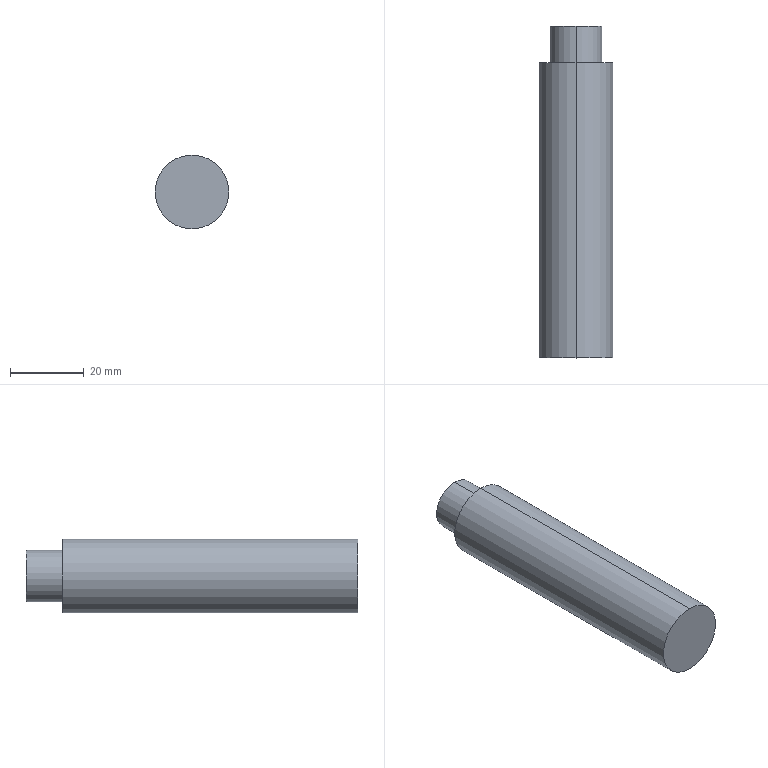Part | SolidWorks | features ICE 4, Extrusion 1, MirrorPattern 1 | 1 solid | 7 faces | box 20 x 90 x 20 mm | volume 26672 mm3 | cylinder 4 | plane 3 | commonest cylinder face diameters 14 x2 20 x2
STEP:
#1=CARTESIAN_POINT('',(0.,90.,7.));
#2=VERTEX_POINT('',#1);
#3=CARTESIAN_POINT('',(0.,90.,-7.));
#4=VERTEX_POINT('',#3);
#5=CARTESIAN_POINT('',(0.,90.,0.));
#6=DIRECTION('',(0.,1.,0.));
#7=DIRECTION('',(0.,0.,1.));
#8=AXIS2_PLACEMENT_3D('',#5,#6,#7);
#9=CIRCLE('',#8,7.);
#10=EDGE_CURVE('',#2,#4,#9,.T.);
#11=ORIENTED_EDGE('',*,*,#10,.F.);
#12=CARTESIAN_POINT('',(0.,80.,7.));
#13=VERTEX_POINT('',#12);
#14=CARTESIAN_POINT('',(0.,90.,7.));
#15=DIRECTION('',(0.,-1.,0.));
#16=VECTOR('',#15,1000.);
#17=LINE('',#14,#16);
#18=EDGE_CURVE('',#2,#13,#17,.T.);
#19=ORIENTED_EDGE('',*,*,#18,.T.);
#20=CARTESIAN_POINT('',(0.,80.,-7.));
#21=VERTEX_POINT('',#20);
#22=CARTESIAN_POINT('',(0.,80.,0.));
#23=DIRECTION('',(0.,1.,0.));
#24=DIRECTION('',(0.,0.,1.));
#25=AXIS2_PLACEMENT_3D('',#22,#23,#24);
#26=CIRCLE('',#25,7.);
#27=EDGE_CURVE('',#13,#21,#26,.T.);
#28=ORIENTED_EDGE('',*,*,#27,.T.);
#29=CARTESIAN_POINT('',(0.,90.,-7.));
#30=DIRECTION('',(0.,-1.,0.));
#31=VECTOR('',#30,1000.);
#32=LINE('',#29,#31);
#33=EDGE_CURVE('',#4,#21,#32,.T.);
#34=ORIENTED_EDGE('',*,*,#33,.F.);
#35=EDGE_LOOP('',(#11,#19,#28,#34));
#36=FACE_OUTER_BOUND('',#35,.T.);
#37=CARTESIAN_POINT('',(0.,90.,0.));
#38=DIRECTION('',(0.,-1.,0.));
#39=DIRECTION('',(0.,0.,-1.));
#40=AXIS2_PLACEMENT_3D('',#37,#38,#39);
#41=CYLINDRICAL_SURFACE('',#40,7.);
#42=ADVANCED_FACE('',(#36),#41,.T.);
#43=CARTESIAN_POINT('',(0.,80.,10.));
#44=VERTEX_POINT('',#43);
#45=CARTESIAN_POINT('',(0.,80.,-10.));
#46=VERTEX_POINT('',#45);
#47=CARTESIAN_POINT('',(0.,80.,0.));
#48=DIRECTION('',(0.,1.,0.));
#49=DIRECTION('',(0.,0.,1.));
#50=AXIS2_PLACEMENT_3D('',#47,#48,#49);
#51=CIRCLE('',#50,10.);
#52=EDGE_CURVE('',#44,#46,#51,.T.);
#53=ORIENTED_EDGE('',*,*,#52,.F.);
#54=CARTESIAN_POINT('',(0.,0.,10.));
#55=VERTEX_POINT('',#54);
#56=CARTESIAN_POINT('',(0.,5.,10.));
#57=DIRECTION('',(0.,-1.,0.));
#58=VECTOR('',#57,1000.);
#59=LINE('',#56,#58);
#60=EDGE_CURVE('',#44,#55,#59,.T.);
#61=ORIENTED_EDGE('',*,*,#60,.T.);
#62=CARTESIAN_POINT('',(0.,0.,-10.));
#63=VERTEX_POINT('',#62);
#64=CARTESIAN_POINT('',(0.,0.,0.));
#65=DIRECTION('',(0.,1.,0.));
#66=DIRECTION('',(0.,0.,1.));
#67=AXIS2_PLACEMENT_3D('',#64,#65,#66);
#68=CIRCLE('',#67,10.);
#69=EDGE_CURVE('',#55,#63,#68,.T.);
#70=ORIENTED_EDGE('',*,*,#69,.T.);
#71=CARTESIAN_POINT('',(0.,5.,-10.));
#72=DIRECTION('',(0.,-1.,0.));
#73=VECTOR('',#72,1000.);
#74=LINE('',#71,#73);
#75=EDGE_CURVE('',#46,#63,#74,.T.);
#76=ORIENTED_EDGE('',*,*,#75,.F.);
#77=EDGE_LOOP('',(#53,#61,#70,#76));
#78=FACE_OUTER_BOUND('',#77,.T.);
#79=CARTESIAN_POINT('',(0.,5.,0.));
#80=DIRECTION('',(0.,-1.,0.));
#81=DIRECTION('',(0.,0.,-1.));
#82=AXIS2_PLACEMENT_3D('',#79,#80,#81);
#83=CYLINDRICAL_SURFACE('',#82,10.);
#84=ADVANCED_FACE('',(#78),#83,.T.);
#85=ORIENTED_EDGE('',*,*,#60,.F.);
#86=CARTESIAN_POINT('',(0.,80.,0.));
#87=DIRECTION('',(0.,1.,0.));
#88=DIRECTION('',(0.,0.,1.));
#89=AXIS2_PLACEMENT_3D('',#86,#87,#88);
#90=CIRCLE('',#89,10.);
#91=EDGE_CURVE('',#46,#44,#90,.T.);
#92=ORIENTED_EDGE('',*,*,#91,.F.);
#93=ORIENTED_EDGE('',*,*,#75,.T.);
#94=CARTESIAN_POINT('',(0.,0.,0.));
#95=DIRECTION('',(0.,1.,0.));
#96=DIRECTION('',(0.,0.,1.));
#97=AXIS2_PLACEMENT_3D('',#94,#95,#96);
#98=CIRCLE('',#97,10.);
#99=EDGE_CURVE('',#63,#55,#98,.T.);
#100=ORIENTED_EDGE('',*,*,#99,.T.);
#101=EDGE_LOOP('',(#85,#92,#93,#100));
#102=FACE_OUTER_BOUND('',#101,.T.);
#103=CARTESIAN_POINT('',(0.,5.,0.));
#104=DIRECTION('',(0.,-1.,0.));
#105=DIRECTION('',(0.,0.,-1.));
#106=AXIS2_PLACEMENT_3D('',#103,#104,#105);
#107=CYLINDRICAL_SURFACE('',#106,10.);
#108=ADVANCED_FACE('',(#102),#107,.T.);
#109=ORIENTED_EDGE('',*,*,#99,.F.);
#110=ORIENTED_EDGE('',*,*,#69,.F.);
#111=EDGE_LOOP('',(#109,#110));
#112=FACE_OUTER_BOUND('',#111,.T.);
#113=CARTESIAN_POINT('',(0.,0.,0.));
#114=DIRECTION('',(0.,1.,0.));
#115=DIRECTION('',(0.,0.,1.));
#116=AXIS2_PLACEMENT_3D('',#113,#114,#115);
#117=PLANE('',#116);
#118=ADVANCED_FACE('',(#112),#117,.F.);
#119=CARTESIAN_POINT('',(0.,80.,0.));
#120=DIRECTION('',(0.,1.,0.));
#121=DIRECTION('',(0.,0.,1.));
#122=AXIS2_PLACEMENT_3D('',#119,#120,#121);
#123=CIRCLE('',#122,7.);
#124=EDGE_CURVE('',#21,#13,#123,.T.);
#125=ORIENTED_EDGE('',*,*,#124,.F.);
#126=ORIENTED_EDGE('',*,*,#27,.F.);
#127=EDGE_LOOP('',(#125,#126));
#128=FACE_BOUND('',#127,.T.);
#129=ORIENTED_EDGE('',*,*,#91,.T.);
#130=ORIENTED_EDGE('',*,*,#52,.T.);
#131=EDGE_LOOP('',(#129,#130));
#132=FACE_OUTER_BOUND('',#131,.T.);
#133=CARTESIAN_POINT('',(0.,80.,0.));
#134=DIRECTION('',(0.,1.,0.));
#135=DIRECTION('',(0.,0.,1.));
#136=AXIS2_PLACEMENT_3D('',#133,#134,#135);
#137=PLANE('',#136);
#138=ADVANCED_FACE('',(#128,#132),#137,.T.);
#139=ORIENTED_EDGE('',*,*,#18,.F.);
#140=CARTESIAN_POINT('',(0.,90.,0.));
#141=DIRECTION('',(0.,1.,0.));
#142=DIRECTION('',(0.,0.,1.));
#143=AXIS2_PLACEMENT_3D('',#140,#141,#142);
#144=CIRCLE('',#143,7.);
#145=EDGE_CURVE('',#4,#2,#144,.T.);
#146=ORIENTED_EDGE('',*,*,#145,.F.);
#147=ORIENTED_EDGE('',*,*,#33,.T.);
#148=ORIENTED_EDGE('',*,*,#124,.T.);
#149=EDGE_LOOP('',(#139,#146,#147,#148));
#150=FACE_OUTER_BOUND('',#149,.T.);
#151=CARTESIAN_POINT('',(0.,90.,0.));
#152=DIRECTION('',(0.,-1.,0.));
#153=DIRECTION('',(0.,0.,-1.));
#154=AXIS2_PLACEMENT_3D('',#151,#152,#153);
#155=CYLINDRICAL_SURFACE('',#154,7.);
#156=ADVANCED_FACE('',(#150),#155,.T.);
#157=ORIENTED_EDGE('',*,*,#145,.T.);
#158=ORIENTED_EDGE('',*,*,#10,.T.);
#159=EDGE_LOOP('',(#157,#158));
#160=FACE_OUTER_BOUND('',#159,.T.);
#161=CARTESIAN_POINT('',(0.,90.,0.));
#162=DIRECTION('',(0.,1.,0.));
#163=DIRECTION('',(0.,0.,1.));
#164=AXIS2_PLACEMENT_3D('',#161,#162,#163);
#165=PLANE('',#164);
#166=ADVANCED_FACE('',(#160),#165,.T.);
#167=CLOSED_SHELL('',(#42,#84,#108,#118,#138,#156,#166));
#168=MANIFOLD_SOLID_BREP('',#167);
#169=CARTESIAN_POINT('',(0.,0.,0.));
#170=DIRECTION('',(0.,0.,1.));
#171=DIRECTION('',(1.,0.,0.));
#172=AXIS2_PLACEMENT_3D('',#169,#170,#171);
#173=(LENGTH_UNIT()NAMED_UNIT(*)SI_UNIT(.MILLI.,.METRE.));
#174=UNCERTAINTY_MEASURE_WITH_UNIT(LENGTH_MEASURE(0.00001),#173,'','');
#175=(NAMED_UNIT(*)PLANE_ANGLE_UNIT()SI_UNIT($,.RADIAN.));
#176=(NAMED_UNIT(*)SI_UNIT($,.STERADIAN.)SOLID_ANGLE_UNIT());
#177=(GEOMETRIC_REPRESENTATION_CONTEXT(3)GLOBAL_UNCERTAINTY_ASSIGNED_CONTEXT((#174))GLOBAL_UNIT_ASSIGNED_CONTEXT((#173,#175,#176))REPRESENTATION_CONTEXT('',''));
#178=ADVANCED_BREP_SHAPE_REPRESENTATION('',(#168,#172),#177);